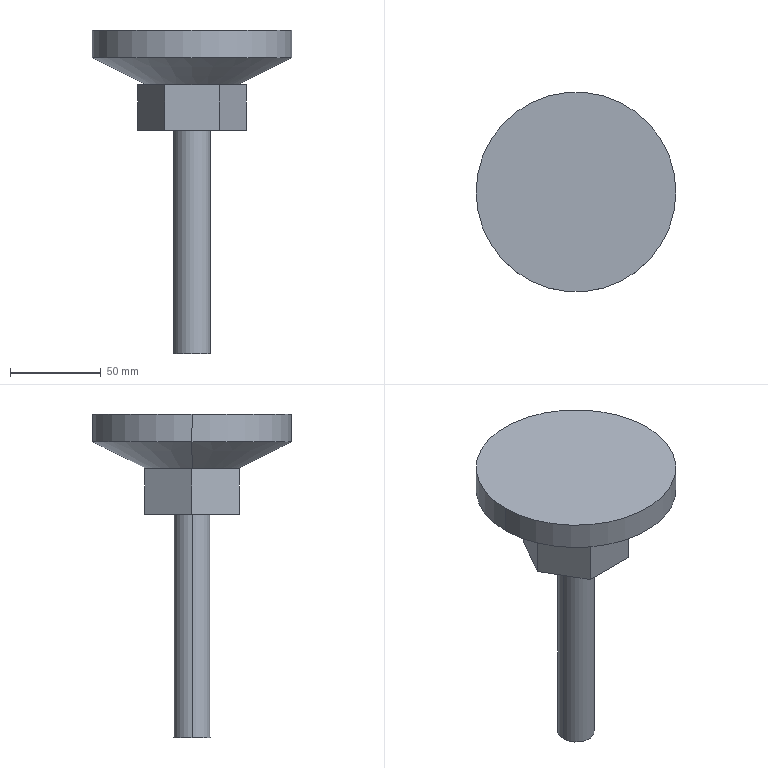Part | SolidWorks | features ICE 2, MirrorPattern 1, RevCut 1, Revolution 1 | 1 solid | 16 faces | box 110 x 110 x 178 mm | volume 318581 mm3 | plane 10 | cylinder 4 | cone 2 | commonest cylinder face diameters 20 x2 110 x2
STEP:
#1=CARTESIAN_POINT('',(10.,0.,83.));
#2=VERTEX_POINT('',#1);
#3=CARTESIAN_POINT('',(-10.,0.,83.));
#4=VERTEX_POINT('',#3);
#5=CARTESIAN_POINT('',(0.,0.,83.));
#6=DIRECTION('',(0.,0.,1.));
#7=DIRECTION('',(-1.,0.,0.));
#8=AXIS2_PLACEMENT_3D('',#5,#6,#7);
#9=CIRCLE('',#8,10.);
#10=EDGE_CURVE('',#2,#4,#9,.T.);
#11=ORIENTED_EDGE('',*,*,#10,.F.);
#12=CARTESIAN_POINT('',(10.,0.,-40.));
#13=VERTEX_POINT('',#12);
#14=CARTESIAN_POINT('',(10.,0.,-40.));
#15=DIRECTION('',(0.,0.,-1.));
#16=VECTOR('',#15,1000.);
#17=LINE('',#14,#16);
#18=EDGE_CURVE('',#2,#13,#17,.T.);
#19=ORIENTED_EDGE('',*,*,#18,.T.);
#20=CARTESIAN_POINT('',(-10.,0.,-40.));
#21=VERTEX_POINT('',#20);
#22=CARTESIAN_POINT('',(0.,0.,-40.));
#23=DIRECTION('',(0.,0.,-1.));
#24=DIRECTION('',(-1.,0.,0.));
#25=AXIS2_PLACEMENT_3D('',#22,#23,#24);
#26=CIRCLE('',#25,10.);
#27=EDGE_CURVE('',#21,#13,#26,.T.);
#28=ORIENTED_EDGE('',*,*,#27,.F.);
#29=CARTESIAN_POINT('',(-10.,0.,-40.));
#30=DIRECTION('',(0.,0.,-1.));
#31=VECTOR('',#30,1000.);
#32=LINE('',#29,#31);
#33=EDGE_CURVE('',#4,#21,#32,.T.);
#34=ORIENTED_EDGE('',*,*,#33,.F.);
#35=EDGE_LOOP('',(#11,#19,#28,#34));
#36=FACE_OUTER_BOUND('',#35,.T.);
#37=CARTESIAN_POINT('',(0.,0.,-40.));
#38=DIRECTION('',(0.,0.,-1.));
#39=DIRECTION('',(-1.,0.,0.));
#40=AXIS2_PLACEMENT_3D('',#37,#38,#39);
#41=CYLINDRICAL_SURFACE('',#40,10.);
#42=ADVANCED_FACE('',(#36),#41,.T.);
#43=CARTESIAN_POINT('',(55.,0.,138.));
#44=VERTEX_POINT('',#43);
#45=CARTESIAN_POINT('',(-55.,0.,138.));
#46=VERTEX_POINT('',#45);
#47=CARTESIAN_POINT('',(0.,0.,138.));
#48=DIRECTION('',(0.,0.,1.));
#49=DIRECTION('',(1.,0.,0.));
#50=AXIS2_PLACEMENT_3D('',#47,#48,#49);
#51=CIRCLE('',#50,55.);
#52=EDGE_CURVE('',#44,#46,#51,.T.);
#53=ORIENTED_EDGE('',*,*,#52,.F.);
#54=CARTESIAN_POINT('',(55.,0.,123.));
#55=VERTEX_POINT('',#54);
#56=CARTESIAN_POINT('',(55.,0.,138.));
#57=DIRECTION('',(0.,0.,-1.));
#58=VECTOR('',#57,1000.);
#59=LINE('',#56,#58);
#60=EDGE_CURVE('',#44,#55,#59,.T.);
#61=ORIENTED_EDGE('',*,*,#60,.T.);
#62=CARTESIAN_POINT('',(-55.,0.,123.));
#63=VERTEX_POINT('',#62);
#64=CARTESIAN_POINT('',(0.,0.,123.));
#65=DIRECTION('',(0.,0.,1.));
#66=DIRECTION('',(1.,0.,0.));
#67=AXIS2_PLACEMENT_3D('',#64,#65,#66);
#68=CIRCLE('',#67,55.);
#69=EDGE_CURVE('',#55,#63,#68,.T.);
#70=ORIENTED_EDGE('',*,*,#69,.T.);
#71=CARTESIAN_POINT('',(-55.,0.,138.));
#72=DIRECTION('',(0.,0.,-1.));
#73=VECTOR('',#72,1000.);
#74=LINE('',#71,#73);
#75=EDGE_CURVE('',#46,#63,#74,.T.);
#76=ORIENTED_EDGE('',*,*,#75,.F.);
#77=EDGE_LOOP('',(#53,#61,#70,#76));
#78=FACE_OUTER_BOUND('',#77,.T.);
#79=CARTESIAN_POINT('',(0.,0.,138.));
#80=DIRECTION('',(0.,0.,-1.));
#81=DIRECTION('',(-1.,0.,0.));
#82=AXIS2_PLACEMENT_3D('',#79,#80,#81);
#83=CYLINDRICAL_SURFACE('',#82,55.);
#84=ADVANCED_FACE('',(#78),#83,.T.);
#85=CARTESIAN_POINT('',(-25.,0.,108.));
#86=VERTEX_POINT('',#85);
#87=CARTESIAN_POINT('',(25.,0.,108.));
#88=VERTEX_POINT('',#87);
#89=CARTESIAN_POINT('',(0.,0.,108.));
#90=DIRECTION('',(0.,0.,-1.));
#91=DIRECTION('',(-1.,0.,0.));
#92=AXIS2_PLACEMENT_3D('',#89,#90,#91);
#93=CIRCLE('',#92,25.);
#94=EDGE_CURVE('',#86,#88,#93,.T.);
#95=ORIENTED_EDGE('',*,*,#94,.F.);
#96=CARTESIAN_POINT('',(-25.,0.,108.));
#97=DIRECTION('',(-0.8944,0.,0.4472));
#98=VECTOR('',#97,1000.);
#99=LINE('',#96,#98);
#100=EDGE_CURVE('',#86,#63,#99,.T.);
#101=ORIENTED_EDGE('',*,*,#100,.T.);
#102=ORIENTED_EDGE('',*,*,#69,.F.);
#103=CARTESIAN_POINT('',(25.,0.,108.));
#104=DIRECTION('',(0.8944,0.,0.4472));
#105=VECTOR('',#104,1000.);
#106=LINE('',#103,#105);
#107=EDGE_CURVE('',#88,#55,#106,.T.);
#108=ORIENTED_EDGE('',*,*,#107,.F.);
#109=EDGE_LOOP('',(#95,#101,#102,#108));
#110=FACE_OUTER_BOUND('',#109,.T.);
#111=CARTESIAN_POINT('',(0.,0.,108.));
#112=DIRECTION('',(0.,0.,1.));
#113=DIRECTION('',(1.,0.,0.));
#114=AXIS2_PLACEMENT_3D('',#111,#112,#113);
#115=CONICAL_SURFACE('',#114,25.,1.107);
#116=ADVANCED_FACE('',(#110),#115,.T.);
#117=ORIENTED_EDGE('',*,*,#100,.F.);
#118=CARTESIAN_POINT('',(0.,0.,108.));
#119=DIRECTION('',(0.,0.,-1.));
#120=DIRECTION('',(-1.,0.,0.));
#121=AXIS2_PLACEMENT_3D('',#118,#119,#120);
#122=CIRCLE('',#121,25.);
#123=EDGE_CURVE('',#88,#86,#122,.T.);
#124=ORIENTED_EDGE('',*,*,#123,.F.);
#125=ORIENTED_EDGE('',*,*,#107,.T.);
#126=CARTESIAN_POINT('',(0.,0.,123.));
#127=DIRECTION('',(0.,0.,1.));
#128=DIRECTION('',(1.,0.,0.));
#129=AXIS2_PLACEMENT_3D('',#126,#127,#128);
#130=CIRCLE('',#129,55.);
#131=EDGE_CURVE('',#63,#55,#130,.T.);
#132=ORIENTED_EDGE('',*,*,#131,.F.);
#133=EDGE_LOOP('',(#117,#124,#125,#132));
#134=FACE_OUTER_BOUND('',#133,.T.);
#135=CARTESIAN_POINT('',(0.,0.,108.));
#136=DIRECTION('',(0.,0.,1.));
#137=DIRECTION('',(1.,0.,0.));
#138=AXIS2_PLACEMENT_3D('',#135,#136,#137);
#139=CONICAL_SURFACE('',#138,25.,1.107);
#140=ADVANCED_FACE('',(#134),#139,.T.);
#141=ORIENTED_EDGE('',*,*,#60,.F.);
#142=CARTESIAN_POINT('',(0.,0.,138.));
#143=DIRECTION('',(0.,0.,1.));
#144=DIRECTION('',(1.,0.,0.));
#145=AXIS2_PLACEMENT_3D('',#142,#143,#144);
#146=CIRCLE('',#145,55.);
#147=EDGE_CURVE('',#46,#44,#146,.T.);
#148=ORIENTED_EDGE('',*,*,#147,.F.);
#149=ORIENTED_EDGE('',*,*,#75,.T.);
#150=ORIENTED_EDGE('',*,*,#131,.T.);
#151=EDGE_LOOP('',(#141,#148,#149,#150));
#152=FACE_OUTER_BOUND('',#151,.T.);
#153=CARTESIAN_POINT('',(0.,0.,138.));
#154=DIRECTION('',(0.,0.,-1.));
#155=DIRECTION('',(-1.,0.,0.));
#156=AXIS2_PLACEMENT_3D('',#153,#154,#155);
#157=CYLINDRICAL_SURFACE('',#156,55.);
#158=ADVANCED_FACE('',(#152),#157,.T.);
#159=ORIENTED_EDGE('',*,*,#147,.T.);
#160=ORIENTED_EDGE('',*,*,#52,.T.);
#161=EDGE_LOOP('',(#159,#160));
#162=FACE_OUTER_BOUND('',#161,.T.);
#163=CARTESIAN_POINT('',(0.,0.,138.));
#164=DIRECTION('',(0.,0.,1.));
#165=DIRECTION('',(1.,0.,0.));
#166=AXIS2_PLACEMENT_3D('',#163,#164,#165);
#167=PLANE('',#166);
#168=ADVANCED_FACE('',(#162),#167,.T.);
#169=CARTESIAN_POINT('',(-30.,0.,108.));
#170=VERTEX_POINT('',#169);
#171=CARTESIAN_POINT('',(-15.,25.981,108.));
#172=VERTEX_POINT('',#171);
#173=CARTESIAN_POINT('',(-30.,0.,108.));
#174=DIRECTION('',(0.5,0.866,0.));
#175=VECTOR('',#174,1000.);
#176=LINE('',#173,#175);
#177=EDGE_CURVE('',#170,#172,#176,.T.);
#178=ORIENTED_EDGE('',*,*,#177,.T.);
#179=CARTESIAN_POINT('',(-15.,25.981,83.));
#180=VERTEX_POINT('',#179);
#181=CARTESIAN_POINT('',(-15.,25.981,83.));
#182=DIRECTION('',(0.,0.,1.));
#183=VECTOR('',#182,1000.);
#184=LINE('',#181,#183);
#185=EDGE_CURVE('',#180,#172,#184,.T.);
#186=ORIENTED_EDGE('',*,*,#185,.F.);
#187=CARTESIAN_POINT('',(-30.,0.,83.));
#188=VERTEX_POINT('',#187);
#189=CARTESIAN_POINT('',(-30.,0.,83.));
#190=DIRECTION('',(0.5,0.866,0.));
#191=VECTOR('',#190,1000.);
#192=LINE('',#189,#191);
#193=EDGE_CURVE('',#188,#180,#192,.T.);
#194=ORIENTED_EDGE('',*,*,#193,.F.);
#195=CARTESIAN_POINT('',(-30.,0.,83.));
#196=DIRECTION('',(0.,0.,1.));
#197=VECTOR('',#196,1000.);
#198=LINE('',#195,#197);
#199=EDGE_CURVE('',#188,#170,#198,.T.);
#200=ORIENTED_EDGE('',*,*,#199,.T.);
#201=EDGE_LOOP('',(#178,#186,#194,#200));
#202=FACE_OUTER_BOUND('',#201,.T.);
#203=CARTESIAN_POINT('',(-30.,0.,83.));
#204=DIRECTION('',(0.866,-0.5,0.));
#205=DIRECTION('',(0.5,0.866,0.));
#206=AXIS2_PLACEMENT_3D('',#203,#204,#205);
#207=PLANE('',#206);
#208=ADVANCED_FACE('',(#202),#207,.F.);
#209=CARTESIAN_POINT('',(15.,25.981,108.));
#210=VERTEX_POINT('',#209);
#211=CARTESIAN_POINT('',(-15.,25.981,108.));
#212=DIRECTION('',(1.,0.,0.));
#213=VECTOR('',#212,1000.);
#214=LINE('',#211,#213);
#215=EDGE_CURVE('',#172,#210,#214,.T.);
#216=ORIENTED_EDGE('',*,*,#215,.T.);
#217=CARTESIAN_POINT('',(15.,25.981,83.));
#218=VERTEX_POINT('',#217);
#219=CARTESIAN_POINT('',(15.,25.981,83.));
#220=DIRECTION('',(0.,0.,1.));
#221=VECTOR('',#220,1000.);
#222=LINE('',#219,#221);
#223=EDGE_CURVE('',#218,#210,#222,.T.);
#224=ORIENTED_EDGE('',*,*,#223,.F.);
#225=CARTESIAN_POINT('',(-15.,25.981,83.));
#226=DIRECTION('',(1.,0.,0.));
#227=VECTOR('',#226,1000.);
#228=LINE('',#225,#227);
#229=EDGE_CURVE('',#180,#218,#228,.T.);
#230=ORIENTED_EDGE('',*,*,#229,.F.);
#231=ORIENTED_EDGE('',*,*,#185,.T.);
#232=EDGE_LOOP('',(#216,#224,#230,#231));
#233=FACE_OUTER_BOUND('',#232,.T.);
#234=CARTESIAN_POINT('',(-15.,25.981,83.));
#235=DIRECTION('',(0.,-1.,0.));
#236=DIRECTION('',(1.,0.,0.));
#237=AXIS2_PLACEMENT_3D('',#234,#235,#236);
#238=PLANE('',#237);
#239=ADVANCED_FACE('',(#233),#238,.F.);
#240=CARTESIAN_POINT('',(30.,0.,108.));
#241=VERTEX_POINT('',#240);
#242=CARTESIAN_POINT('',(15.,25.981,108.));
#243=DIRECTION('',(0.5,-0.866,0.));
#244=VECTOR('',#243,1000.);
#245=LINE('',#242,#244);
#246=EDGE_CURVE('',#210,#241,#245,.T.);
#247=ORIENTED_EDGE('',*,*,#246,.T.);
#248=CARTESIAN_POINT('',(30.,0.,83.));
#249=VERTEX_POINT('',#248);
#250=CARTESIAN_POINT('',(30.,0.,83.));
#251=DIRECTION('',(0.,0.,1.));
#252=VECTOR('',#251,1000.);
#253=LINE('',#250,#252);
#254=EDGE_CURVE('',#249,#241,#253,.T.);
#255=ORIENTED_EDGE('',*,*,#254,.F.);
#256=CARTESIAN_POINT('',(15.,25.981,83.));
#257=DIRECTION('',(0.5,-0.866,0.));
#258=VECTOR('',#257,1000.);
#259=LINE('',#256,#258);
#260=EDGE_CURVE('',#218,#249,#259,.T.);
#261=ORIENTED_EDGE('',*,*,#260,.F.);
#262=ORIENTED_EDGE('',*,*,#223,.T.);
#263=EDGE_LOOP('',(#247,#255,#261,#262));
#264=FACE_OUTER_BOUND('',#263,.T.);
#265=CARTESIAN_POINT('',(15.,25.981,83.));
#266=DIRECTION('',(-0.866,-0.5,0.));
#267=DIRECTION('',(0.5,-0.866,0.));
#268=AXIS2_PLACEMENT_3D('',#265,#266,#267);
#269=PLANE('',#268);
#270=ADVANCED_FACE('',(#264),#269,.F.);
#271=CARTESIAN_POINT('',(15.,-25.981,108.));
#272=VERTEX_POINT('',#271);
#273=CARTESIAN_POINT('',(30.,0.,108.));
#274=DIRECTION('',(-0.5,-0.866,0.));
#275=VECTOR('',#274,1000.);
#276=LINE('',#273,#275);
#277=EDGE_CURVE('',#241,#272,#276,.T.);
#278=ORIENTED_EDGE('',*,*,#277,.T.);
#279=CARTESIAN_POINT('',(15.,-25.981,83.));
#280=VERTEX_POINT('',#279);
#281=CARTESIAN_POINT('',(15.,-25.981,83.));
#282=DIRECTION('',(0.,0.,1.));
#283=VECTOR('',#282,1000.);
#284=LINE('',#281,#283);
#285=EDGE_CURVE('',#280,#272,#284,.T.);
#286=ORIENTED_EDGE('',*,*,#285,.F.);
#287=CARTESIAN_POINT('',(30.,0.,83.));
#288=DIRECTION('',(-0.5,-0.866,0.));
#289=VECTOR('',#288,1000.);
#290=LINE('',#287,#289);
#291=EDGE_CURVE('',#249,#280,#290,.T.);
#292=ORIENTED_EDGE('',*,*,#291,.F.);
#293=ORIENTED_EDGE('',*,*,#254,.T.);
#294=EDGE_LOOP('',(#278,#286,#292,#293));
#295=FACE_OUTER_BOUND('',#294,.T.);
#296=CARTESIAN_POINT('',(30.,0.,83.));
#297=DIRECTION('',(-0.866,0.5,0.));
#298=DIRECTION('',(-0.5,-0.866,0.));
#299=AXIS2_PLACEMENT_3D('',#296,#297,#298);
#300=PLANE('',#299);
#301=ADVANCED_FACE('',(#295),#300,.F.);
#302=CARTESIAN_POINT('',(-15.,-25.981,108.));
#303=VERTEX_POINT('',#302);
#304=CARTESIAN_POINT('',(15.,-25.981,108.));
#305=DIRECTION('',(-1.,0.,0.));
#306=VECTOR('',#305,1000.);
#307=LINE('',#304,#306);
#308=EDGE_CURVE('',#272,#303,#307,.T.);
#309=ORIENTED_EDGE('',*,*,#308,.T.);
#310=CARTESIAN_POINT('',(-15.,-25.981,83.));
#311=VERTEX_POINT('',#310);
#312=CARTESIAN_POINT('',(-15.,-25.981,83.));
#313=DIRECTION('',(0.,0.,1.));
#314=VECTOR('',#313,1000.);
#315=LINE('',#312,#314);
#316=EDGE_CURVE('',#311,#303,#315,.T.);
#317=ORIENTED_EDGE('',*,*,#316,.F.);
#318=CARTESIAN_POINT('',(15.,-25.981,83.));
#319=DIRECTION('',(-1.,0.,0.));
#320=VECTOR('',#319,1000.);
#321=LINE('',#318,#320);
#322=EDGE_CURVE('',#280,#311,#321,.T.);
#323=ORIENTED_EDGE('',*,*,#322,.F.);
#324=ORIENTED_EDGE('',*,*,#285,.T.);
#325=EDGE_LOOP('',(#309,#317,#323,#324));
#326=FACE_OUTER_BOUND('',#325,.T.);
#327=CARTESIAN_POINT('',(15.,-25.981,83.));
#328=DIRECTION('',(0.,1.,0.));
#329=DIRECTION('',(-1.,0.,0.));
#330=AXIS2_PLACEMENT_3D('',#327,#328,#329);
#331=PLANE('',#330);
#332=ADVANCED_FACE('',(#326),#331,.F.);
#333=CARTESIAN_POINT('',(-15.,-25.981,108.));
#334=DIRECTION('',(-0.5,0.866,0.));
#335=VECTOR('',#334,1000.);
#336=LINE('',#333,#335);
#337=EDGE_CURVE('',#303,#170,#336,.T.);
#338=ORIENTED_EDGE('',*,*,#337,.T.);
#339=ORIENTED_EDGE('',*,*,#199,.F.);
#340=CARTESIAN_POINT('',(-15.,-25.981,83.));
#341=DIRECTION('',(-0.5,0.866,0.));
#342=VECTOR('',#341,1000.);
#343=LINE('',#340,#342);
#344=EDGE_CURVE('',#311,#188,#343,.T.);
#345=ORIENTED_EDGE('',*,*,#344,.F.);
#346=ORIENTED_EDGE('',*,*,#316,.T.);
#347=EDGE_LOOP('',(#338,#339,#345,#346));
#348=FACE_OUTER_BOUND('',#347,.T.);
#349=CARTESIAN_POINT('',(-15.,-25.981,83.));
#350=DIRECTION('',(0.866,0.5,0.));
#351=DIRECTION('',(-0.5,0.866,0.));
#352=AXIS2_PLACEMENT_3D('',#349,#350,#351);
#353=PLANE('',#352);
#354=ADVANCED_FACE('',(#348),#353,.F.);
#355=CARTESIAN_POINT('',(0.,0.,83.));
#356=DIRECTION('',(0.,0.,1.));
#357=DIRECTION('',(-1.,0.,0.));
#358=AXIS2_PLACEMENT_3D('',#355,#356,#357);
#359=CIRCLE('',#358,10.);
#360=EDGE_CURVE('',#4,#2,#359,.T.);
#361=ORIENTED_EDGE('',*,*,#360,.T.);
#362=ORIENTED_EDGE('',*,*,#10,.T.);
#363=EDGE_LOOP('',(#361,#362));
#364=FACE_BOUND('',#363,.T.);
#365=ORIENTED_EDGE('',*,*,#193,.T.);
#366=ORIENTED_EDGE('',*,*,#229,.T.);
#367=ORIENTED_EDGE('',*,*,#260,.T.);
#368=ORIENTED_EDGE('',*,*,#291,.T.);
#369=ORIENTED_EDGE('',*,*,#322,.T.);
#370=ORIENTED_EDGE('',*,*,#344,.T.);
#371=EDGE_LOOP('',(#365,#366,#367,#368,#369,#370));
#372=FACE_OUTER_BOUND('',#371,.T.);
#373=CARTESIAN_POINT('',(0.,0.,83.));
#374=DIRECTION('',(0.,0.,-1.));
#375=DIRECTION('',(-1.,0.,0.));
#376=AXIS2_PLACEMENT_3D('',#373,#374,#375);
#377=PLANE('',#376);
#378=ADVANCED_FACE('',(#364,#372),#377,.T.);
#379=ORIENTED_EDGE('',*,*,#123,.T.);
#380=ORIENTED_EDGE('',*,*,#94,.T.);
#381=EDGE_LOOP('',(#379,#380));
#382=FACE_BOUND('',#381,.T.);
#383=ORIENTED_EDGE('',*,*,#177,.F.);
#384=ORIENTED_EDGE('',*,*,#337,.F.);
#385=ORIENTED_EDGE('',*,*,#308,.F.);
#386=ORIENTED_EDGE('',*,*,#277,.F.);
#387=ORIENTED_EDGE('',*,*,#246,.F.);
#388=ORIENTED_EDGE('',*,*,#215,.F.);
#389=EDGE_LOOP('',(#383,#384,#385,#386,#387,#388));
#390=FACE_OUTER_BOUND('',#389,.T.);
#391=CARTESIAN_POINT('',(0.,0.,108.));
#392=DIRECTION('',(0.,0.,-1.));
#393=DIRECTION('',(-1.,0.,0.));
#394=AXIS2_PLACEMENT_3D('',#391,#392,#393);
#395=PLANE('',#394);
#396=ADVANCED_FACE('',(#382,#390),#395,.F.);
#397=ORIENTED_EDGE('',*,*,#27,.T.);
#398=CARTESIAN_POINT('',(0.,0.,-40.));
#399=DIRECTION('',(0.,0.,-1.));
#400=DIRECTION('',(-1.,0.,0.));
#401=AXIS2_PLACEMENT_3D('',#398,#399,#400);
#402=CIRCLE('',#401,10.);
#403=EDGE_CURVE('',#13,#21,#402,.T.);
#404=ORIENTED_EDGE('',*,*,#403,.T.);
#405=EDGE_LOOP('',(#397,#404));
#406=FACE_OUTER_BOUND('',#405,.T.);
#407=CARTESIAN_POINT('',(0.,0.,-40.));
#408=DIRECTION('',(0.,0.,-1.));
#409=DIRECTION('',(-1.,0.,0.));
#410=AXIS2_PLACEMENT_3D('',#407,#408,#409);
#411=PLANE('',#410);
#412=ADVANCED_FACE('',(#406),#411,.T.);
#413=ORIENTED_EDGE('',*,*,#18,.F.);
#414=ORIENTED_EDGE('',*,*,#360,.F.);
#415=ORIENTED_EDGE('',*,*,#33,.T.);
#416=ORIENTED_EDGE('',*,*,#403,.F.);
#417=EDGE_LOOP('',(#413,#414,#415,#416));
#418=FACE_OUTER_BOUND('',#417,.T.);
#419=CARTESIAN_POINT('',(0.,0.,-40.));
#420=DIRECTION('',(0.,0.,-1.));
#421=DIRECTION('',(-1.,0.,0.));
#422=AXIS2_PLACEMENT_3D('',#419,#420,#421);
#423=CYLINDRICAL_SURFACE('',#422,10.);
#424=ADVANCED_FACE('',(#418),#423,.T.);
#425=CLOSED_SHELL('',(#42,#84,#116,#140,#158,#168,#208,#239,#270,#301,#332,#354,#378,#396,#412,#424));
#426=MANIFOLD_SOLID_BREP('',#425);
#427=CARTESIAN_POINT('',(0.,0.,0.));
#428=DIRECTION('',(0.,0.,1.));
#429=DIRECTION('',(1.,0.,0.));
#430=AXIS2_PLACEMENT_3D('',#427,#428,#429);
#431=(LENGTH_UNIT()NAMED_UNIT(*)SI_UNIT(.MILLI.,.METRE.));
#432=UNCERTAINTY_MEASURE_WITH_UNIT(LENGTH_MEASURE(0.00001),#431,'','');
#433=(NAMED_UNIT(*)PLANE_ANGLE_UNIT()SI_UNIT($,.RADIAN.));
#434=(NAMED_UNIT(*)SI_UNIT($,.STERADIAN.)SOLID_ANGLE_UNIT());
#435=(GEOMETRIC_REPRESENTATION_CONTEXT(3)GLOBAL_UNCERTAINTY_ASSIGNED_CONTEXT((#432))GLOBAL_UNIT_ASSIGNED_CONTEXT((#431,#433,#434))REPRESENTATION_CONTEXT('',''));
#436=ADVANCED_BREP_SHAPE_REPRESENTATION('',(#426,#430),#435);